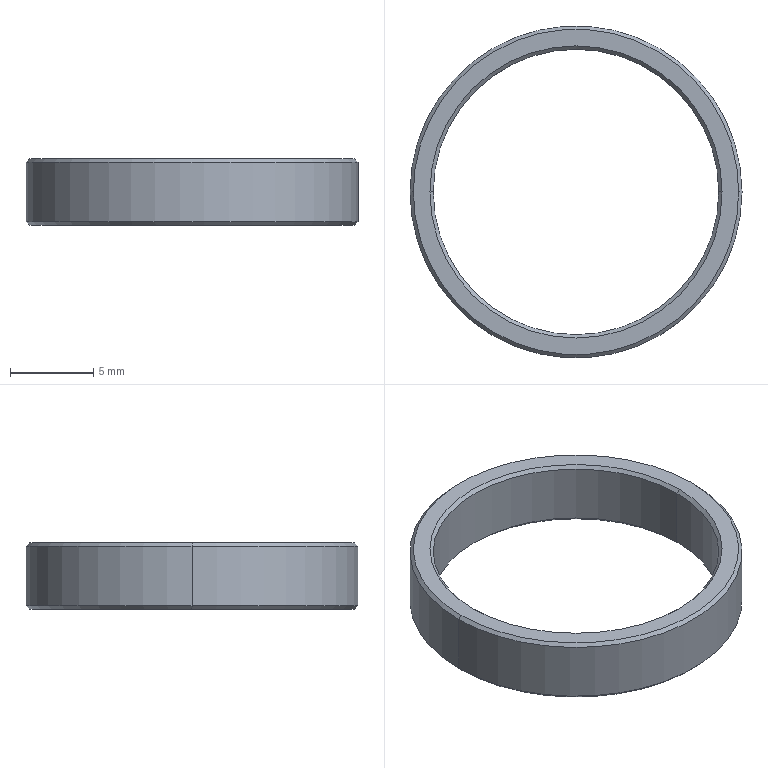Part | NX | features BREP 1 | 1 solid | 14 faces | box 20 x 20 x 4 mm | volume 322.554 mm3 | cone 8 | cylinder 4 | plane 2 | commonest cylinder face diameters 17.2 x2 20 x2
STEP:
#1=CARTESIAN_POINT('',(-8.6,0.,1.8));
#2=VERTEX_POINT('',#1);
#3=CARTESIAN_POINT('',(8.6,0.,1.8));
#4=VERTEX_POINT('',#3);
#5=CARTESIAN_POINT('',(0.,0.,1.8));
#6=DIRECTION('',(0.,0.,1.));
#7=DIRECTION('',(1.,0.,0.));
#8=AXIS2_PLACEMENT_3D('',#5,#6,#7);
#9=CIRCLE('',#8,8.6);
#10=EDGE_CURVE('',#2,#4,#9,.T.);
#11=ORIENTED_EDGE('',*,*,#10,.F.);
#12=CARTESIAN_POINT('',(-8.8,0.,2.));
#13=VERTEX_POINT('',#12);
#14=CARTESIAN_POINT('',(-8.6,0.,1.8));
#15=DIRECTION('',(-0.7071,0.,0.7071));
#16=VECTOR('',#15,1000.);
#17=LINE('',#14,#16);
#18=EDGE_CURVE('',#13,#2,#17,.F.);
#19=ORIENTED_EDGE('',*,*,#18,.F.);
#20=CARTESIAN_POINT('',(8.8,0.,2.));
#21=VERTEX_POINT('',#20);
#22=CARTESIAN_POINT('',(0.,0.,2.));
#23=DIRECTION('',(0.,0.,-1.));
#24=DIRECTION('',(1.,0.,0.));
#25=AXIS2_PLACEMENT_3D('',#22,#23,#24);
#26=CIRCLE('',#25,8.8);
#27=EDGE_CURVE('',#21,#13,#26,.T.);
#28=ORIENTED_EDGE('',*,*,#27,.F.);
#29=CARTESIAN_POINT('',(8.6,0.,1.8));
#30=DIRECTION('',(0.7071,0.,0.7071));
#31=VECTOR('',#30,1000.);
#32=LINE('',#29,#31);
#33=EDGE_CURVE('',#21,#4,#32,.F.);
#34=ORIENTED_EDGE('',*,*,#33,.T.);
#35=EDGE_LOOP('',(#11,#19,#28,#34));
#36=FACE_BOUND('',#35,.T.);
#37=CARTESIAN_POINT('',(0.,0.,1.8));
#38=DIRECTION('',(0.,0.,1.));
#39=DIRECTION('',(1.,0.,0.));
#40=AXIS2_PLACEMENT_3D('',#37,#38,#39);
#41=CONICAL_SURFACE('',#40,8.6,0.7854);
#42=ADVANCED_FACE('',(#36),#41,.F.);
#43=CARTESIAN_POINT('',(8.6,0.,-1.8));
#44=VERTEX_POINT('',#43);
#45=CARTESIAN_POINT('',(-8.6,0.,-1.8));
#46=VERTEX_POINT('',#45);
#47=CARTESIAN_POINT('',(0.,0.,-1.8));
#48=DIRECTION('',(0.,0.,-1.));
#49=DIRECTION('',(1.,0.,0.));
#50=AXIS2_PLACEMENT_3D('',#47,#48,#49);
#51=CIRCLE('',#50,8.6);
#52=EDGE_CURVE('',#44,#46,#51,.T.);
#53=ORIENTED_EDGE('',*,*,#52,.F.);
#54=CARTESIAN_POINT('',(8.8,0.,-2.));
#55=VERTEX_POINT('',#54);
#56=CARTESIAN_POINT('',(8.8,0.,-2.));
#57=DIRECTION('',(0.7071,0.,-0.7071));
#58=VECTOR('',#57,1000.);
#59=LINE('',#56,#58);
#60=EDGE_CURVE('',#44,#55,#59,.T.);
#61=ORIENTED_EDGE('',*,*,#60,.T.);
#62=CARTESIAN_POINT('',(-8.8,0.,-2.));
#63=VERTEX_POINT('',#62);
#64=CARTESIAN_POINT('',(0.,0.,-2.));
#65=DIRECTION('',(0.,0.,1.));
#66=DIRECTION('',(1.,0.,0.));
#67=AXIS2_PLACEMENT_3D('',#64,#65,#66);
#68=CIRCLE('',#67,8.8);
#69=EDGE_CURVE('',#63,#55,#68,.T.);
#70=ORIENTED_EDGE('',*,*,#69,.F.);
#71=CARTESIAN_POINT('',(-8.8,0.,-2.));
#72=DIRECTION('',(-0.7071,0.,-0.7071));
#73=VECTOR('',#72,1000.);
#74=LINE('',#71,#73);
#75=EDGE_CURVE('',#46,#63,#74,.T.);
#76=ORIENTED_EDGE('',*,*,#75,.F.);
#77=EDGE_LOOP('',(#53,#61,#70,#76));
#78=FACE_BOUND('',#77,.T.);
#79=CARTESIAN_POINT('',(0.,0.,-2.));
#80=DIRECTION('',(0.,0.,-1.));
#81=DIRECTION('',(-1.,0.,0.));
#82=AXIS2_PLACEMENT_3D('',#79,#80,#81);
#83=CONICAL_SURFACE('',#82,8.8,0.7854);
#84=ADVANCED_FACE('',(#78),#83,.F.);
#85=CARTESIAN_POINT('',(-9.8,0.,-2.));
#86=VERTEX_POINT('',#85);
#87=CARTESIAN_POINT('',(9.8,0.,-2.));
#88=VERTEX_POINT('',#87);
#89=CARTESIAN_POINT('',(0.,0.,-2.));
#90=DIRECTION('',(0.,0.,-1.));
#91=DIRECTION('',(1.,0.,0.));
#92=AXIS2_PLACEMENT_3D('',#89,#90,#91);
#93=CIRCLE('',#92,9.8);
#94=EDGE_CURVE('',#86,#88,#93,.T.);
#95=ORIENTED_EDGE('',*,*,#94,.F.);
#96=CARTESIAN_POINT('',(-10.,0.,-1.8));
#97=VERTEX_POINT('',#96);
#98=CARTESIAN_POINT('',(-10.,0.,-1.8));
#99=DIRECTION('',(-0.7071,0.,0.7071));
#100=VECTOR('',#99,1000.);
#101=LINE('',#98,#100);
#102=EDGE_CURVE('',#97,#86,#101,.F.);
#103=ORIENTED_EDGE('',*,*,#102,.F.);
#104=CARTESIAN_POINT('',(10.,0.,-1.8));
#105=VERTEX_POINT('',#104);
#106=CARTESIAN_POINT('',(0.,0.,-1.8));
#107=DIRECTION('',(0.,0.,1.));
#108=DIRECTION('',(1.,0.,0.));
#109=AXIS2_PLACEMENT_3D('',#106,#107,#108);
#110=CIRCLE('',#109,10.);
#111=EDGE_CURVE('',#105,#97,#110,.T.);
#112=ORIENTED_EDGE('',*,*,#111,.F.);
#113=CARTESIAN_POINT('',(10.,0.,-1.8));
#114=DIRECTION('',(0.7071,0.,0.7071));
#115=VECTOR('',#114,1000.);
#116=LINE('',#113,#115);
#117=EDGE_CURVE('',#105,#88,#116,.F.);
#118=ORIENTED_EDGE('',*,*,#117,.T.);
#119=EDGE_LOOP('',(#95,#103,#112,#118));
#120=FACE_BOUND('',#119,.T.);
#121=CARTESIAN_POINT('',(0.,0.,-1.8));
#122=DIRECTION('',(0.,0.,1.));
#123=DIRECTION('',(1.,0.,0.));
#124=AXIS2_PLACEMENT_3D('',#121,#122,#123);
#125=CONICAL_SURFACE('',#124,10.,0.7854);
#126=ADVANCED_FACE('',(#120),#125,.T.);
#127=CARTESIAN_POINT('',(9.8,0.,2.));
#128=VERTEX_POINT('',#127);
#129=CARTESIAN_POINT('',(-9.8,0.,2.));
#130=VERTEX_POINT('',#129);
#131=CARTESIAN_POINT('',(0.,0.,2.));
#132=DIRECTION('',(0.,0.,1.));
#133=DIRECTION('',(1.,0.,0.));
#134=AXIS2_PLACEMENT_3D('',#131,#132,#133);
#135=CIRCLE('',#134,9.8);
#136=EDGE_CURVE('',#128,#130,#135,.T.);
#137=ORIENTED_EDGE('',*,*,#136,.F.);
#138=CARTESIAN_POINT('',(10.,0.,1.8));
#139=VERTEX_POINT('',#138);
#140=CARTESIAN_POINT('',(9.8,0.,2.));
#141=DIRECTION('',(0.7071,0.,-0.7071));
#142=VECTOR('',#141,1000.);
#143=LINE('',#140,#142);
#144=EDGE_CURVE('',#128,#139,#143,.T.);
#145=ORIENTED_EDGE('',*,*,#144,.T.);
#146=CARTESIAN_POINT('',(-10.,0.,1.8));
#147=VERTEX_POINT('',#146);
#148=CARTESIAN_POINT('',(0.,0.,1.8));
#149=DIRECTION('',(0.,0.,-1.));
#150=DIRECTION('',(1.,0.,0.));
#151=AXIS2_PLACEMENT_3D('',#148,#149,#150);
#152=CIRCLE('',#151,10.);
#153=EDGE_CURVE('',#147,#139,#152,.T.);
#154=ORIENTED_EDGE('',*,*,#153,.F.);
#155=CARTESIAN_POINT('',(-9.8,0.,2.));
#156=DIRECTION('',(-0.7071,0.,-0.7071));
#157=VECTOR('',#156,1000.);
#158=LINE('',#155,#157);
#159=EDGE_CURVE('',#130,#147,#158,.T.);
#160=ORIENTED_EDGE('',*,*,#159,.F.);
#161=EDGE_LOOP('',(#137,#145,#154,#160));
#162=FACE_BOUND('',#161,.T.);
#163=CARTESIAN_POINT('',(0.,0.,2.));
#164=DIRECTION('',(0.,0.,-1.));
#165=DIRECTION('',(-1.,0.,0.));
#166=AXIS2_PLACEMENT_3D('',#163,#164,#165);
#167=CONICAL_SURFACE('',#166,9.8,0.7854);
#168=ADVANCED_FACE('',(#162),#167,.T.);
#169=ORIENTED_EDGE('',*,*,#10,.T.);
#170=CARTESIAN_POINT('',(8.6,0.,2.));
#171=DIRECTION('',(0.,0.,-1.));
#172=VECTOR('',#171,1000.);
#173=LINE('',#170,#172);
#174=EDGE_CURVE('',#4,#44,#173,.T.);
#175=ORIENTED_EDGE('',*,*,#174,.T.);
#176=ORIENTED_EDGE('',*,*,#52,.T.);
#177=CARTESIAN_POINT('',(-8.6,0.,2.));
#178=DIRECTION('',(0.,0.,-1.));
#179=VECTOR('',#178,1000.);
#180=LINE('',#177,#179);
#181=EDGE_CURVE('',#2,#46,#180,.T.);
#182=ORIENTED_EDGE('',*,*,#181,.F.);
#183=EDGE_LOOP('',(#169,#175,#176,#182));
#184=FACE_BOUND('',#183,.T.);
#185=CARTESIAN_POINT('',(0.,0.,2.));
#186=DIRECTION('',(0.,0.,-1.));
#187=DIRECTION('',(-1.,0.,0.));
#188=AXIS2_PLACEMENT_3D('',#185,#186,#187);
#189=CYLINDRICAL_SURFACE('',#188,8.6);
#190=ADVANCED_FACE('',(#184),#189,.F.);
#191=ORIENTED_EDGE('',*,*,#153,.T.);
#192=CARTESIAN_POINT('',(10.,0.,2.));
#193=DIRECTION('',(0.,0.,-1.));
#194=VECTOR('',#193,1000.);
#195=LINE('',#192,#194);
#196=EDGE_CURVE('',#139,#105,#195,.T.);
#197=ORIENTED_EDGE('',*,*,#196,.T.);
#198=ORIENTED_EDGE('',*,*,#111,.T.);
#199=CARTESIAN_POINT('',(-10.,0.,2.));
#200=DIRECTION('',(0.,0.,-1.));
#201=VECTOR('',#200,1000.);
#202=LINE('',#199,#201);
#203=EDGE_CURVE('',#147,#97,#202,.T.);
#204=ORIENTED_EDGE('',*,*,#203,.F.);
#205=EDGE_LOOP('',(#191,#197,#198,#204));
#206=FACE_BOUND('',#205,.T.);
#207=CARTESIAN_POINT('',(0.,0.,2.));
#208=DIRECTION('',(0.,0.,-1.));
#209=DIRECTION('',(-1.,0.,0.));
#210=AXIS2_PLACEMENT_3D('',#207,#208,#209);
#211=CYLINDRICAL_SURFACE('',#210,10.);
#212=ADVANCED_FACE('',(#206),#211,.T.);
#213=CARTESIAN_POINT('',(0.,0.,2.));
#214=DIRECTION('',(0.,0.,1.));
#215=DIRECTION('',(1.,0.,0.));
#216=AXIS2_PLACEMENT_3D('',#213,#214,#215);
#217=CIRCLE('',#216,9.8);
#218=EDGE_CURVE('',#130,#128,#217,.T.);
#219=ORIENTED_EDGE('',*,*,#218,.T.);
#220=ORIENTED_EDGE('',*,*,#136,.T.);
#221=EDGE_LOOP('',(#219,#220));
#222=FACE_BOUND('',#221,.T.);
#223=ORIENTED_EDGE('',*,*,#27,.T.);
#224=CARTESIAN_POINT('',(0.,0.,2.));
#225=DIRECTION('',(0.,0.,-1.));
#226=DIRECTION('',(1.,0.,0.));
#227=AXIS2_PLACEMENT_3D('',#224,#225,#226);
#228=CIRCLE('',#227,8.8);
#229=EDGE_CURVE('',#13,#21,#228,.T.);
#230=ORIENTED_EDGE('',*,*,#229,.T.);
#231=EDGE_LOOP('',(#223,#230));
#232=FACE_BOUND('',#231,.T.);
#233=CARTESIAN_POINT('',(0.,0.,2.));
#234=DIRECTION('',(0.,0.,1.));
#235=DIRECTION('',(1.,0.,0.));
#236=AXIS2_PLACEMENT_3D('',#233,#234,#235);
#237=PLANE('',#236);
#238=ADVANCED_FACE('',(#222,#232),#237,.T.);
#239=CARTESIAN_POINT('',(0.,0.,-2.));
#240=DIRECTION('',(0.,0.,-1.));
#241=DIRECTION('',(1.,0.,0.));
#242=AXIS2_PLACEMENT_3D('',#239,#240,#241);
#243=CIRCLE('',#242,9.8);
#244=EDGE_CURVE('',#88,#86,#243,.T.);
#245=ORIENTED_EDGE('',*,*,#244,.T.);
#246=ORIENTED_EDGE('',*,*,#94,.T.);
#247=EDGE_LOOP('',(#245,#246));
#248=FACE_BOUND('',#247,.T.);
#249=ORIENTED_EDGE('',*,*,#69,.T.);
#250=CARTESIAN_POINT('',(0.,0.,-2.));
#251=DIRECTION('',(0.,0.,1.));
#252=DIRECTION('',(1.,0.,0.));
#253=AXIS2_PLACEMENT_3D('',#250,#251,#252);
#254=CIRCLE('',#253,8.8);
#255=EDGE_CURVE('',#55,#63,#254,.T.);
#256=ORIENTED_EDGE('',*,*,#255,.T.);
#257=EDGE_LOOP('',(#249,#256));
#258=FACE_BOUND('',#257,.T.);
#259=CARTESIAN_POINT('',(0.,0.,-2.));
#260=DIRECTION('',(0.,0.,1.));
#261=DIRECTION('',(1.,0.,0.));
#262=AXIS2_PLACEMENT_3D('',#259,#260,#261);
#263=PLANE('',#262);
#264=ADVANCED_FACE('',(#248,#258),#263,.F.);
#265=ORIENTED_EDGE('',*,*,#196,.F.);
#266=CARTESIAN_POINT('',(0.,0.,1.8));
#267=DIRECTION('',(0.,0.,-1.));
#268=DIRECTION('',(1.,0.,0.));
#269=AXIS2_PLACEMENT_3D('',#266,#267,#268);
#270=CIRCLE('',#269,10.);
#271=EDGE_CURVE('',#139,#147,#270,.T.);
#272=ORIENTED_EDGE('',*,*,#271,.T.);
#273=ORIENTED_EDGE('',*,*,#203,.T.);
#274=CARTESIAN_POINT('',(0.,0.,-1.8));
#275=DIRECTION('',(0.,0.,1.));
#276=DIRECTION('',(1.,0.,0.));
#277=AXIS2_PLACEMENT_3D('',#274,#275,#276);
#278=CIRCLE('',#277,10.);
#279=EDGE_CURVE('',#97,#105,#278,.T.);
#280=ORIENTED_EDGE('',*,*,#279,.T.);
#281=EDGE_LOOP('',(#265,#272,#273,#280));
#282=FACE_BOUND('',#281,.T.);
#283=CARTESIAN_POINT('',(0.,0.,2.));
#284=DIRECTION('',(0.,0.,-1.));
#285=DIRECTION('',(-1.,0.,0.));
#286=AXIS2_PLACEMENT_3D('',#283,#284,#285);
#287=CYLINDRICAL_SURFACE('',#286,10.);
#288=ADVANCED_FACE('',(#282),#287,.T.);
#289=ORIENTED_EDGE('',*,*,#174,.F.);
#290=CARTESIAN_POINT('',(0.,0.,1.8));
#291=DIRECTION('',(0.,0.,1.));
#292=DIRECTION('',(1.,0.,0.));
#293=AXIS2_PLACEMENT_3D('',#290,#291,#292);
#294=CIRCLE('',#293,8.6);
#295=EDGE_CURVE('',#4,#2,#294,.T.);
#296=ORIENTED_EDGE('',*,*,#295,.T.);
#297=ORIENTED_EDGE('',*,*,#181,.T.);
#298=CARTESIAN_POINT('',(0.,0.,-1.8));
#299=DIRECTION('',(0.,0.,-1.));
#300=DIRECTION('',(1.,0.,0.));
#301=AXIS2_PLACEMENT_3D('',#298,#299,#300);
#302=CIRCLE('',#301,8.6);
#303=EDGE_CURVE('',#46,#44,#302,.T.);
#304=ORIENTED_EDGE('',*,*,#303,.T.);
#305=EDGE_LOOP('',(#289,#296,#297,#304));
#306=FACE_BOUND('',#305,.T.);
#307=CARTESIAN_POINT('',(0.,0.,2.));
#308=DIRECTION('',(0.,0.,-1.));
#309=DIRECTION('',(-1.,0.,0.));
#310=AXIS2_PLACEMENT_3D('',#307,#308,#309);
#311=CYLINDRICAL_SURFACE('',#310,8.6);
#312=ADVANCED_FACE('',(#306),#311,.F.);
#313=ORIENTED_EDGE('',*,*,#144,.F.);
#314=ORIENTED_EDGE('',*,*,#218,.F.);
#315=ORIENTED_EDGE('',*,*,#159,.T.);
#316=ORIENTED_EDGE('',*,*,#271,.F.);
#317=EDGE_LOOP('',(#313,#314,#315,#316));
#318=FACE_BOUND('',#317,.T.);
#319=CARTESIAN_POINT('',(0.,0.,2.));
#320=DIRECTION('',(0.,0.,-1.));
#321=DIRECTION('',(-1.,0.,0.));
#322=AXIS2_PLACEMENT_3D('',#319,#320,#321);
#323=CONICAL_SURFACE('',#322,9.8,0.7854);
#324=ADVANCED_FACE('',(#318),#323,.T.);
#325=ORIENTED_EDGE('',*,*,#102,.T.);
#326=ORIENTED_EDGE('',*,*,#244,.F.);
#327=ORIENTED_EDGE('',*,*,#117,.F.);
#328=ORIENTED_EDGE('',*,*,#279,.F.);
#329=EDGE_LOOP('',(#325,#326,#327,#328));
#330=FACE_BOUND('',#329,.T.);
#331=CARTESIAN_POINT('',(0.,0.,-1.8));
#332=DIRECTION('',(0.,0.,1.));
#333=DIRECTION('',(1.,0.,0.));
#334=AXIS2_PLACEMENT_3D('',#331,#332,#333);
#335=CONICAL_SURFACE('',#334,10.,0.7854);
#336=ADVANCED_FACE('',(#330),#335,.T.);
#337=ORIENTED_EDGE('',*,*,#60,.F.);
#338=ORIENTED_EDGE('',*,*,#303,.F.);
#339=ORIENTED_EDGE('',*,*,#75,.T.);
#340=ORIENTED_EDGE('',*,*,#255,.F.);
#341=EDGE_LOOP('',(#337,#338,#339,#340));
#342=FACE_BOUND('',#341,.T.);
#343=CARTESIAN_POINT('',(0.,0.,-2.));
#344=DIRECTION('',(0.,0.,-1.));
#345=DIRECTION('',(-1.,0.,0.));
#346=AXIS2_PLACEMENT_3D('',#343,#344,#345);
#347=CONICAL_SURFACE('',#346,8.8,0.7854);
#348=ADVANCED_FACE('',(#342),#347,.F.);
#349=ORIENTED_EDGE('',*,*,#18,.T.);
#350=ORIENTED_EDGE('',*,*,#295,.F.);
#351=ORIENTED_EDGE('',*,*,#33,.F.);
#352=ORIENTED_EDGE('',*,*,#229,.F.);
#353=EDGE_LOOP('',(#349,#350,#351,#352));
#354=FACE_BOUND('',#353,.T.);
#355=CARTESIAN_POINT('',(0.,0.,1.8));
#356=DIRECTION('',(0.,0.,1.));
#357=DIRECTION('',(1.,0.,0.));
#358=AXIS2_PLACEMENT_3D('',#355,#356,#357);
#359=CONICAL_SURFACE('',#358,8.6,0.7854);
#360=ADVANCED_FACE('',(#354),#359,.F.);
#361=CLOSED_SHELL('',(#42,#84,#126,#168,#190,#212,#238,#264,#288,#312,#324,#336,#348,#360));
#362=MANIFOLD_SOLID_BREP('',#361);
#363=(LENGTH_UNIT()NAMED_UNIT(*)SI_UNIT(.MILLI.,.METRE.));
#364=UNCERTAINTY_MEASURE_WITH_UNIT(LENGTH_MEASURE(0.00001),#363,'','');
#365=(NAMED_UNIT(*)PLANE_ANGLE_UNIT()SI_UNIT($,.RADIAN.));
#366=(NAMED_UNIT(*)SI_UNIT($,.STERADIAN.)SOLID_ANGLE_UNIT());
#367=(GEOMETRIC_REPRESENTATION_CONTEXT(3)GLOBAL_UNCERTAINTY_ASSIGNED_CONTEXT((#364))GLOBAL_UNIT_ASSIGNED_CONTEXT((#363,#365,#366))REPRESENTATION_CONTEXT('',''));
#368=ADVANCED_BREP_SHAPE_REPRESENTATION('',(#362),#367);